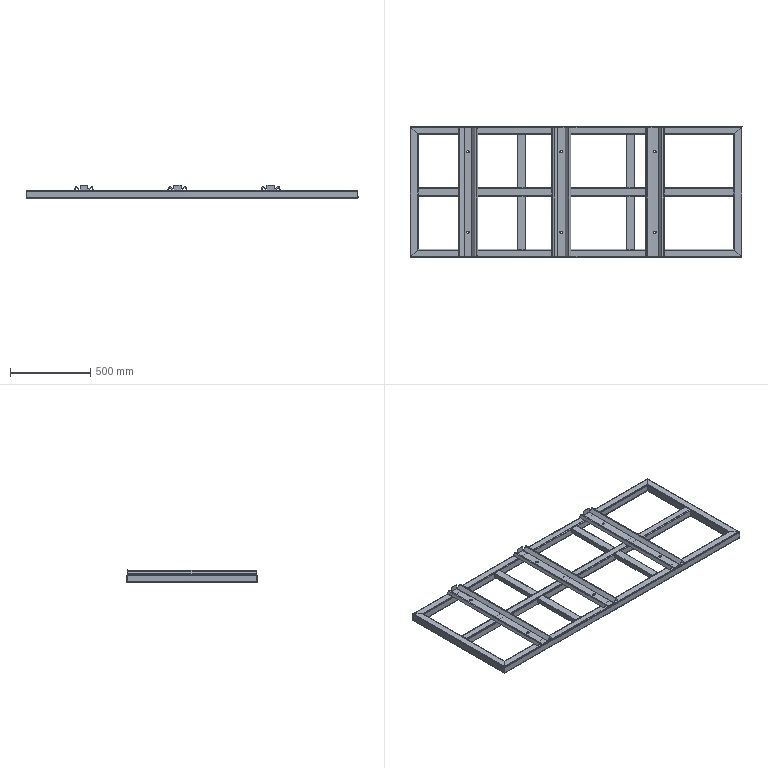Part | SolidWorks | 12 solids | 358 faces | box 2070 x 815 x 84 mm | volume 5892624 mm3 | plane 242 | cylinder 116 | commonest cylinder face diameters 6 x20 12 x20 10 x18 13 x18 0.2 x17 8.2 x9